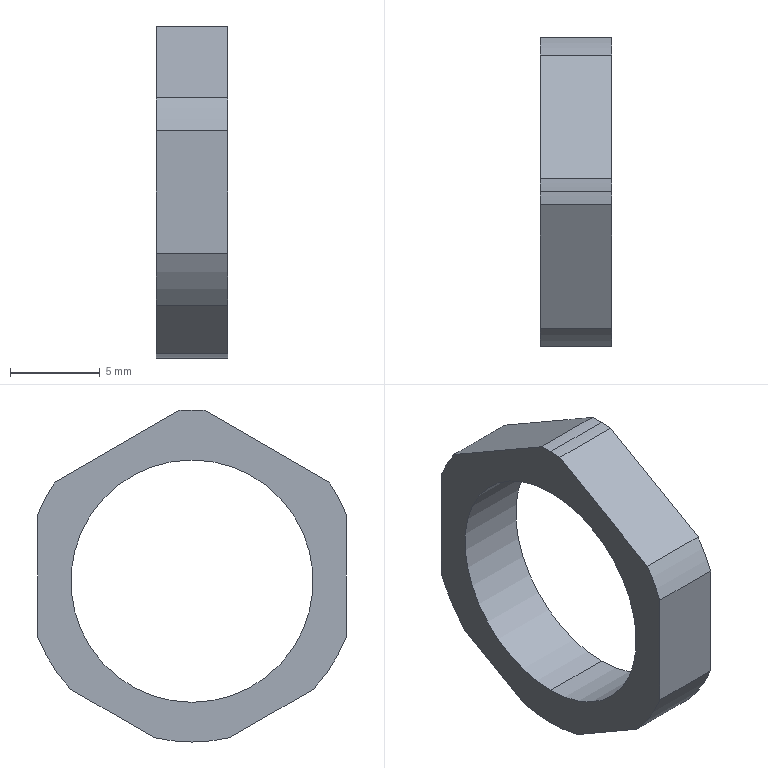Part | SolidWorks | features BaseBody 1 | 1 solid | 17 faces | box 4 x 17.2 x 18.5 mm | volume 428.753 mm3 | cylinder 9 | plane 8 | commonest cylinder face diameters 18.5 x7 13.5 x2
STEP:
#1=CARTESIAN_POINT('',(325.,17.5,16.75));
#2=VERTEX_POINT('',#1);
#3=CARTESIAN_POINT('',(325.,17.5,30.25));
#4=VERTEX_POINT('',#3);
#5=CARTESIAN_POINT('',(325.,17.5,23.5));
#6=DIRECTION('',(-1.,0.,0.));
#7=DIRECTION('',(0.,0.,1.));
#8=AXIS2_PLACEMENT_3D('',#5,#6,#7);
#9=CIRCLE('',#8,6.75);
#10=EDGE_CURVE('',#2,#4,#9,.T.);
#11=ORIENTED_EDGE('',*,*,#10,.F.);
#12=CARTESIAN_POINT('',(321.,17.5,16.75));
#13=VERTEX_POINT('',#12);
#14=CARTESIAN_POINT('',(325.,17.5,16.75));
#15=DIRECTION('',(-1.,0.,0.));
#16=VECTOR('',#15,1000.);
#17=LINE('',#14,#16);
#18=EDGE_CURVE('',#2,#13,#17,.T.);
#19=ORIENTED_EDGE('',*,*,#18,.T.);
#20=CARTESIAN_POINT('',(321.,17.5,30.25));
#21=VERTEX_POINT('',#20);
#22=CARTESIAN_POINT('',(321.,17.5,23.5));
#23=DIRECTION('',(-1.,0.,0.));
#24=DIRECTION('',(0.,0.,1.));
#25=AXIS2_PLACEMENT_3D('',#22,#23,#24);
#26=CIRCLE('',#25,6.75);
#27=EDGE_CURVE('',#13,#21,#26,.T.);
#28=ORIENTED_EDGE('',*,*,#27,.T.);
#29=CARTESIAN_POINT('',(325.,17.5,30.25));
#30=DIRECTION('',(-1.,0.,0.));
#31=VECTOR('',#30,1000.);
#32=LINE('',#29,#31);
#33=EDGE_CURVE('',#4,#21,#32,.T.);
#34=ORIENTED_EDGE('',*,*,#33,.F.);
#35=EDGE_LOOP('',(#11,#19,#28,#34));
#36=FACE_OUTER_BOUND('',#35,.T.);
#37=CARTESIAN_POINT('',(325.,17.5,23.5));
#38=DIRECTION('',(-1.,0.,0.));
#39=DIRECTION('',(0.,0.,1.));
#40=AXIS2_PLACEMENT_3D('',#37,#38,#39);
#41=CYLINDRICAL_SURFACE('',#40,6.75);
#42=ADVANCED_FACE('',(#36),#41,.F.);
#43=CARTESIAN_POINT('',(325.,17.5,33.038));
#44=VERTEX_POINT('',#43);
#45=CARTESIAN_POINT('',(325.,16.77,33.009));
#46=VERTEX_POINT('',#45);
#47=CARTESIAN_POINT('',(325.,17.5,23.788));
#48=DIRECTION('',(1.,0.,0.));
#49=DIRECTION('',(0.,0.,1.));
#50=AXIS2_PLACEMENT_3D('',#47,#48,#49);
#51=CIRCLE('',#50,9.25);
#52=EDGE_CURVE('',#44,#46,#51,.T.);
#53=ORIENTED_EDGE('',*,*,#52,.F.);
#54=CARTESIAN_POINT('',(321.,17.5,33.038));
#55=VERTEX_POINT('',#54);
#56=CARTESIAN_POINT('',(325.,17.5,33.038));
#57=DIRECTION('',(-1.,0.,0.));
#58=VECTOR('',#57,1000.);
#59=LINE('',#56,#58);
#60=EDGE_CURVE('',#44,#55,#59,.T.);
#61=ORIENTED_EDGE('',*,*,#60,.T.);
#62=CARTESIAN_POINT('',(321.,16.77,33.009));
#63=VERTEX_POINT('',#62);
#64=CARTESIAN_POINT('',(321.,17.5,23.788));
#65=DIRECTION('',(1.,0.,0.));
#66=DIRECTION('',(0.,0.,1.));
#67=AXIS2_PLACEMENT_3D('',#64,#65,#66);
#68=CIRCLE('',#67,9.25);
#69=EDGE_CURVE('',#55,#63,#68,.T.);
#70=ORIENTED_EDGE('',*,*,#69,.T.);
#71=CARTESIAN_POINT('',(325.,16.77,33.009));
#72=DIRECTION('',(1.,0.,0.));
#73=VECTOR('',#72,1000.);
#74=LINE('',#71,#73);
#75=EDGE_CURVE('',#63,#46,#74,.T.);
#76=ORIENTED_EDGE('',*,*,#75,.T.);
#77=EDGE_LOOP('',(#53,#61,#70,#76));
#78=FACE_OUTER_BOUND('',#77,.T.);
#79=CARTESIAN_POINT('',(325.,17.5,23.788));
#80=DIRECTION('',(-1.,0.,0.));
#81=DIRECTION('',(0.,0.,1.));
#82=AXIS2_PLACEMENT_3D('',#79,#80,#81);
#83=CYLINDRICAL_SURFACE('',#82,9.25);
#84=ADVANCED_FACE('',(#78),#83,.T.);
#85=CARTESIAN_POINT('',(325.,17.5,23.5));
#86=DIRECTION('',(-1.,0.,0.));
#87=DIRECTION('',(0.,0.,1.));
#88=AXIS2_PLACEMENT_3D('',#85,#86,#87);
#89=CIRCLE('',#88,6.75);
#90=EDGE_CURVE('',#4,#2,#89,.T.);
#91=ORIENTED_EDGE('',*,*,#90,.T.);
#92=ORIENTED_EDGE('',*,*,#10,.T.);
#93=EDGE_LOOP('',(#91,#92));
#94=FACE_BOUND('',#93,.T.);
#95=CARTESIAN_POINT('',(325.,25.121,29.03));
#96=VERTEX_POINT('',#95);
#97=CARTESIAN_POINT('',(325.,18.23,33.009));
#98=VERTEX_POINT('',#97);
#99=CARTESIAN_POINT('',(325.,25.121,29.03));
#100=DIRECTION('',(0.,-0.866,0.5));
#101=VECTOR('',#100,1000.);
#102=LINE('',#99,#101);
#103=EDGE_CURVE('',#96,#98,#102,.T.);
#104=ORIENTED_EDGE('',*,*,#103,.T.);
#105=CARTESIAN_POINT('',(325.,17.5,23.788));
#106=DIRECTION('',(1.,0.,0.));
#107=DIRECTION('',(0.,0.,1.));
#108=AXIS2_PLACEMENT_3D('',#105,#106,#107);
#109=CIRCLE('',#108,9.25);
#110=EDGE_CURVE('',#98,#44,#109,.T.);
#111=ORIENTED_EDGE('',*,*,#110,.T.);
#112=ORIENTED_EDGE('',*,*,#52,.T.);
#113=CARTESIAN_POINT('',(325.,9.879,29.03));
#114=VERTEX_POINT('',#113);
#115=CARTESIAN_POINT('',(325.,16.77,33.009));
#116=DIRECTION('',(0.,-0.866,-0.5));
#117=VECTOR('',#116,1000.);
#118=LINE('',#115,#117);
#119=EDGE_CURVE('',#46,#114,#118,.T.);
#120=ORIENTED_EDGE('',*,*,#119,.T.);
#121=CARTESIAN_POINT('',(325.,8.9,27.194));
#122=VERTEX_POINT('',#121);
#123=CARTESIAN_POINT('',(325.,17.5,23.788));
#124=DIRECTION('',(-1.,0.,0.));
#125=DIRECTION('',(0.,0.,1.));
#126=AXIS2_PLACEMENT_3D('',#123,#124,#125);
#127=CIRCLE('',#126,9.25);
#128=EDGE_CURVE('',#122,#114,#127,.T.);
#129=ORIENTED_EDGE('',*,*,#128,.F.);
#130=CARTESIAN_POINT('',(325.,8.9,20.382));
#131=VERTEX_POINT('',#130);
#132=CARTESIAN_POINT('',(325.,8.9,20.382));
#133=DIRECTION('',(0.,0.,1.));
#134=VECTOR('',#133,1000.);
#135=LINE('',#132,#134);
#136=EDGE_CURVE('',#131,#122,#135,.T.);
#137=ORIENTED_EDGE('',*,*,#136,.F.);
#138=CARTESIAN_POINT('',(325.,10.743,17.471));
#139=VERTEX_POINT('',#138);
#140=CARTESIAN_POINT('',(325.,17.5,23.788));
#141=DIRECTION('',(-1.,0.,0.));
#142=DIRECTION('',(0.,0.,1.));
#143=AXIS2_PLACEMENT_3D('',#140,#141,#142);
#144=CIRCLE('',#143,9.25);
#145=EDGE_CURVE('',#139,#131,#144,.T.);
#146=ORIENTED_EDGE('',*,*,#145,.F.);
#147=CARTESIAN_POINT('',(325.,15.407,14.778));
#148=VERTEX_POINT('',#147);
#149=CARTESIAN_POINT('',(325.,10.743,17.471));
#150=DIRECTION('',(0.,0.866,-0.5));
#151=VECTOR('',#150,1000.);
#152=LINE('',#149,#151);
#153=EDGE_CURVE('',#139,#148,#152,.T.);
#154=ORIENTED_EDGE('',*,*,#153,.T.);
#155=CARTESIAN_POINT('',(325.,19.593,14.778));
#156=VERTEX_POINT('',#155);
#157=CARTESIAN_POINT('',(325.,17.5,23.788));
#158=DIRECTION('',(-1.,0.,0.));
#159=DIRECTION('',(0.,0.,1.));
#160=AXIS2_PLACEMENT_3D('',#157,#158,#159);
#161=CIRCLE('',#160,9.25);
#162=EDGE_CURVE('',#156,#148,#161,.T.);
#163=ORIENTED_EDGE('',*,*,#162,.F.);
#164=CARTESIAN_POINT('',(325.,24.257,17.471));
#165=VERTEX_POINT('',#164);
#166=CARTESIAN_POINT('',(325.,19.593,14.778));
#167=DIRECTION('',(0.,0.866,0.5));
#168=VECTOR('',#167,1000.);
#169=LINE('',#166,#168);
#170=EDGE_CURVE('',#156,#165,#169,.T.);
#171=ORIENTED_EDGE('',*,*,#170,.T.);
#172=CARTESIAN_POINT('',(325.,26.1,20.382));
#173=VERTEX_POINT('',#172);
#174=CARTESIAN_POINT('',(325.,17.5,23.788));
#175=DIRECTION('',(-1.,0.,0.));
#176=DIRECTION('',(0.,0.,1.));
#177=AXIS2_PLACEMENT_3D('',#174,#175,#176);
#178=CIRCLE('',#177,9.25);
#179=EDGE_CURVE('',#173,#165,#178,.T.);
#180=ORIENTED_EDGE('',*,*,#179,.F.);
#181=CARTESIAN_POINT('',(325.,26.1,27.194));
#182=VERTEX_POINT('',#181);
#183=CARTESIAN_POINT('',(325.,26.1,27.194));
#184=DIRECTION('',(0.,0.,-1.));
#185=VECTOR('',#184,1000.);
#186=LINE('',#183,#185);
#187=EDGE_CURVE('',#182,#173,#186,.T.);
#188=ORIENTED_EDGE('',*,*,#187,.F.);
#189=CARTESIAN_POINT('',(325.,17.5,23.788));
#190=DIRECTION('',(-1.,0.,0.));
#191=DIRECTION('',(0.,0.,1.));
#192=AXIS2_PLACEMENT_3D('',#189,#190,#191);
#193=CIRCLE('',#192,9.25);
#194=EDGE_CURVE('',#96,#182,#193,.T.);
#195=ORIENTED_EDGE('',*,*,#194,.F.);
#196=EDGE_LOOP('',(#104,#111,#112,#120,#129,#137,#146,#154,#163,#171,#180,#188,#195));
#197=FACE_OUTER_BOUND('',#196,.T.);
#198=CARTESIAN_POINT('',(325.,17.5,23.5));
#199=DIRECTION('',(1.,0.,0.));
#200=DIRECTION('',(0.,1.,0.));
#201=AXIS2_PLACEMENT_3D('',#198,#199,#200);
#202=PLANE('',#201);
#203=ADVANCED_FACE('',(#94,#197),#202,.T.);
#204=CARTESIAN_POINT('',(321.,8.9,20.382));
#205=VERTEX_POINT('',#204);
#206=CARTESIAN_POINT('',(321.,10.743,17.471));
#207=VERTEX_POINT('',#206);
#208=CARTESIAN_POINT('',(321.,17.5,23.788));
#209=DIRECTION('',(1.,0.,0.));
#210=DIRECTION('',(0.,0.,1.));
#211=AXIS2_PLACEMENT_3D('',#208,#209,#210);
#212=CIRCLE('',#211,9.25);
#213=EDGE_CURVE('',#205,#207,#212,.T.);
#214=ORIENTED_EDGE('',*,*,#213,.T.);
#215=CARTESIAN_POINT('',(325.,10.743,17.471));
#216=DIRECTION('',(1.,0.,0.));
#217=VECTOR('',#216,1000.);
#218=LINE('',#215,#217);
#219=EDGE_CURVE('',#207,#139,#218,.T.);
#220=ORIENTED_EDGE('',*,*,#219,.T.);
#221=ORIENTED_EDGE('',*,*,#145,.T.);
#222=CARTESIAN_POINT('',(325.,8.9,20.382));
#223=DIRECTION('',(1.,0.,0.));
#224=VECTOR('',#223,1000.);
#225=LINE('',#222,#224);
#226=EDGE_CURVE('',#205,#131,#225,.T.);
#227=ORIENTED_EDGE('',*,*,#226,.F.);
#228=EDGE_LOOP('',(#214,#220,#221,#227));
#229=FACE_OUTER_BOUND('',#228,.T.);
#230=CARTESIAN_POINT('',(325.,17.5,23.788));
#231=DIRECTION('',(-1.,0.,0.));
#232=DIRECTION('',(0.,0.,1.));
#233=AXIS2_PLACEMENT_3D('',#230,#231,#232);
#234=CYLINDRICAL_SURFACE('',#233,9.25);
#235=ADVANCED_FACE('',(#229),#234,.T.);
#236=ORIENTED_EDGE('',*,*,#153,.F.);
#237=ORIENTED_EDGE('',*,*,#219,.F.);
#238=CARTESIAN_POINT('',(321.,15.407,14.778));
#239=VERTEX_POINT('',#238);
#240=CARTESIAN_POINT('',(321.,10.743,17.471));
#241=DIRECTION('',(0.,0.866,-0.5));
#242=VECTOR('',#241,1000.);
#243=LINE('',#240,#242);
#244=EDGE_CURVE('',#207,#239,#243,.T.);
#245=ORIENTED_EDGE('',*,*,#244,.T.);
#246=CARTESIAN_POINT('',(325.,15.407,14.778));
#247=DIRECTION('',(-1.,0.,0.));
#248=VECTOR('',#247,1000.);
#249=LINE('',#246,#248);
#250=EDGE_CURVE('',#148,#239,#249,.T.);
#251=ORIENTED_EDGE('',*,*,#250,.F.);
#252=EDGE_LOOP('',(#236,#237,#245,#251));
#253=FACE_OUTER_BOUND('',#252,.T.);
#254=CARTESIAN_POINT('',(325.,10.743,17.471));
#255=DIRECTION('',(0.,0.5,0.866));
#256=DIRECTION('',(1.,0.,0.));
#257=AXIS2_PLACEMENT_3D('',#254,#255,#256);
#258=PLANE('',#257);
#259=ADVANCED_FACE('',(#253),#258,.F.);
#260=ORIENTED_EDGE('',*,*,#162,.T.);
#261=ORIENTED_EDGE('',*,*,#250,.T.);
#262=CARTESIAN_POINT('',(321.,19.593,14.778));
#263=VERTEX_POINT('',#262);
#264=CARTESIAN_POINT('',(321.,17.5,23.788));
#265=DIRECTION('',(1.,0.,0.));
#266=DIRECTION('',(0.,0.,1.));
#267=AXIS2_PLACEMENT_3D('',#264,#265,#266);
#268=CIRCLE('',#267,9.25);
#269=EDGE_CURVE('',#239,#263,#268,.T.);
#270=ORIENTED_EDGE('',*,*,#269,.T.);
#271=CARTESIAN_POINT('',(325.,19.593,14.778));
#272=DIRECTION('',(1.,0.,0.));
#273=VECTOR('',#272,1000.);
#274=LINE('',#271,#273);
#275=EDGE_CURVE('',#263,#156,#274,.T.);
#276=ORIENTED_EDGE('',*,*,#275,.T.);
#277=EDGE_LOOP('',(#260,#261,#270,#276));
#278=FACE_OUTER_BOUND('',#277,.T.);
#279=CARTESIAN_POINT('',(325.,17.5,23.788));
#280=DIRECTION('',(-1.,0.,0.));
#281=DIRECTION('',(0.,0.,1.));
#282=AXIS2_PLACEMENT_3D('',#279,#280,#281);
#283=CYLINDRICAL_SURFACE('',#282,9.25);
#284=ADVANCED_FACE('',(#278),#283,.T.);
#285=ORIENTED_EDGE('',*,*,#170,.F.);
#286=ORIENTED_EDGE('',*,*,#275,.F.);
#287=CARTESIAN_POINT('',(321.,24.257,17.471));
#288=VERTEX_POINT('',#287);
#289=CARTESIAN_POINT('',(321.,19.593,14.778));
#290=DIRECTION('',(0.,0.866,0.5));
#291=VECTOR('',#290,1000.);
#292=LINE('',#289,#291);
#293=EDGE_CURVE('',#263,#288,#292,.T.);
#294=ORIENTED_EDGE('',*,*,#293,.T.);
#295=CARTESIAN_POINT('',(325.,24.257,17.471));
#296=DIRECTION('',(-1.,0.,0.));
#297=VECTOR('',#296,1000.);
#298=LINE('',#295,#297);
#299=EDGE_CURVE('',#165,#288,#298,.T.);
#300=ORIENTED_EDGE('',*,*,#299,.F.);
#301=EDGE_LOOP('',(#285,#286,#294,#300));
#302=FACE_OUTER_BOUND('',#301,.T.);
#303=CARTESIAN_POINT('',(325.,19.593,14.778));
#304=DIRECTION('',(0.,-0.5,0.866));
#305=DIRECTION('',(-1.,0.,0.));
#306=AXIS2_PLACEMENT_3D('',#303,#304,#305);
#307=PLANE('',#306);
#308=ADVANCED_FACE('',(#302),#307,.F.);
#309=CARTESIAN_POINT('',(321.,26.1,20.382));
#310=VERTEX_POINT('',#309);
#311=CARTESIAN_POINT('',(321.,17.5,23.788));
#312=DIRECTION('',(1.,0.,0.));
#313=DIRECTION('',(0.,0.,1.));
#314=AXIS2_PLACEMENT_3D('',#311,#312,#313);
#315=CIRCLE('',#314,9.25);
#316=EDGE_CURVE('',#288,#310,#315,.T.);
#317=ORIENTED_EDGE('',*,*,#316,.T.);
#318=CARTESIAN_POINT('',(325.,26.1,20.382));
#319=DIRECTION('',(-1.,0.,0.));
#320=VECTOR('',#319,1000.);
#321=LINE('',#318,#320);
#322=EDGE_CURVE('',#173,#310,#321,.T.);
#323=ORIENTED_EDGE('',*,*,#322,.F.);
#324=ORIENTED_EDGE('',*,*,#179,.T.);
#325=ORIENTED_EDGE('',*,*,#299,.T.);
#326=EDGE_LOOP('',(#317,#323,#324,#325));
#327=FACE_OUTER_BOUND('',#326,.T.);
#328=CARTESIAN_POINT('',(325.,17.5,23.788));
#329=DIRECTION('',(-1.,0.,0.));
#330=DIRECTION('',(0.,0.,1.));
#331=AXIS2_PLACEMENT_3D('',#328,#329,#330);
#332=CYLINDRICAL_SURFACE('',#331,9.25);
#333=ADVANCED_FACE('',(#327),#332,.T.);
#334=CARTESIAN_POINT('',(321.,26.1,27.194));
#335=VERTEX_POINT('',#334);
#336=CARTESIAN_POINT('',(321.,26.1,23.5));
#337=DIRECTION('',(0.,0.,1.));
#338=VECTOR('',#337,1000.);
#339=LINE('',#336,#338);
#340=EDGE_CURVE('',#310,#335,#339,.T.);
#341=ORIENTED_EDGE('',*,*,#340,.T.);
#342=CARTESIAN_POINT('',(325.,26.1,27.194));
#343=DIRECTION('',(-1.,0.,0.));
#344=VECTOR('',#343,1000.);
#345=LINE('',#342,#344);
#346=EDGE_CURVE('',#182,#335,#345,.T.);
#347=ORIENTED_EDGE('',*,*,#346,.F.);
#348=ORIENTED_EDGE('',*,*,#187,.T.);
#349=ORIENTED_EDGE('',*,*,#322,.T.);
#350=EDGE_LOOP('',(#341,#347,#348,#349));
#351=FACE_OUTER_BOUND('',#350,.T.);
#352=CARTESIAN_POINT('',(325.,26.1,27.194));
#353=DIRECTION('',(0.,1.,0.));
#354=DIRECTION('',(1.,0.,0.));
#355=AXIS2_PLACEMENT_3D('',#352,#353,#354);
#356=PLANE('',#355);
#357=ADVANCED_FACE('',(#351),#356,.T.);
#358=CARTESIAN_POINT('',(321.,25.121,29.03));
#359=VERTEX_POINT('',#358);
#360=CARTESIAN_POINT('',(321.,17.5,23.788));
#361=DIRECTION('',(1.,0.,0.));
#362=DIRECTION('',(0.,0.,1.));
#363=AXIS2_PLACEMENT_3D('',#360,#361,#362);
#364=CIRCLE('',#363,9.25);
#365=EDGE_CURVE('',#335,#359,#364,.T.);
#366=ORIENTED_EDGE('',*,*,#365,.T.);
#367=CARTESIAN_POINT('',(325.,25.121,29.03));
#368=DIRECTION('',(1.,0.,0.));
#369=VECTOR('',#368,1000.);
#370=LINE('',#367,#369);
#371=EDGE_CURVE('',#359,#96,#370,.T.);
#372=ORIENTED_EDGE('',*,*,#371,.T.);
#373=ORIENTED_EDGE('',*,*,#194,.T.);
#374=ORIENTED_EDGE('',*,*,#346,.T.);
#375=EDGE_LOOP('',(#366,#372,#373,#374));
#376=FACE_OUTER_BOUND('',#375,.T.);
#377=CARTESIAN_POINT('',(325.,17.5,23.788));
#378=DIRECTION('',(-1.,0.,0.));
#379=DIRECTION('',(0.,0.,1.));
#380=AXIS2_PLACEMENT_3D('',#377,#378,#379);
#381=CYLINDRICAL_SURFACE('',#380,9.25);
#382=ADVANCED_FACE('',(#376),#381,.T.);
#383=ORIENTED_EDGE('',*,*,#103,.F.);
#384=ORIENTED_EDGE('',*,*,#371,.F.);
#385=CARTESIAN_POINT('',(321.,18.23,33.009));
#386=VERTEX_POINT('',#385);
#387=CARTESIAN_POINT('',(321.,25.121,29.03));
#388=DIRECTION('',(0.,-0.866,0.5));
#389=VECTOR('',#388,1000.);
#390=LINE('',#387,#389);
#391=EDGE_CURVE('',#359,#386,#390,.T.);
#392=ORIENTED_EDGE('',*,*,#391,.T.);
#393=CARTESIAN_POINT('',(325.,18.23,33.009));
#394=DIRECTION('',(-1.,0.,0.));
#395=VECTOR('',#394,1000.);
#396=LINE('',#393,#395);
#397=EDGE_CURVE('',#98,#386,#396,.T.);
#398=ORIENTED_EDGE('',*,*,#397,.F.);
#399=EDGE_LOOP('',(#383,#384,#392,#398));
#400=FACE_OUTER_BOUND('',#399,.T.);
#401=CARTESIAN_POINT('',(325.,25.121,29.03));
#402=DIRECTION('',(0.,-0.5,-0.866));
#403=DIRECTION('',(0.,-0.866,0.5));
#404=AXIS2_PLACEMENT_3D('',#401,#402,#403);
#405=PLANE('',#404);
#406=ADVANCED_FACE('',(#400),#405,.F.);
#407=ORIENTED_EDGE('',*,*,#119,.F.);
#408=ORIENTED_EDGE('',*,*,#75,.F.);
#409=CARTESIAN_POINT('',(321.,9.879,29.03));
#410=VERTEX_POINT('',#409);
#411=CARTESIAN_POINT('',(321.,16.77,33.009));
#412=DIRECTION('',(0.,-0.866,-0.5));
#413=VECTOR('',#412,1000.);
#414=LINE('',#411,#413);
#415=EDGE_CURVE('',#63,#410,#414,.T.);
#416=ORIENTED_EDGE('',*,*,#415,.T.);
#417=CARTESIAN_POINT('',(325.,9.879,29.03));
#418=DIRECTION('',(-1.,0.,0.));
#419=VECTOR('',#418,1000.);
#420=LINE('',#417,#419);
#421=EDGE_CURVE('',#114,#410,#420,.T.);
#422=ORIENTED_EDGE('',*,*,#421,.F.);
#423=EDGE_LOOP('',(#407,#408,#416,#422));
#424=FACE_OUTER_BOUND('',#423,.T.);
#425=CARTESIAN_POINT('',(325.,16.77,33.009));
#426=DIRECTION('',(0.,0.5,-0.866));
#427=DIRECTION('',(-1.,0.,0.));
#428=AXIS2_PLACEMENT_3D('',#425,#426,#427);
#429=PLANE('',#428);
#430=ADVANCED_FACE('',(#424),#429,.F.);
#431=CARTESIAN_POINT('',(321.,8.9,27.194));
#432=VERTEX_POINT('',#431);
#433=CARTESIAN_POINT('',(321.,17.5,23.788));
#434=DIRECTION('',(1.,0.,0.));
#435=DIRECTION('',(0.,0.,1.));
#436=AXIS2_PLACEMENT_3D('',#433,#434,#435);
#437=CIRCLE('',#436,9.25);
#438=EDGE_CURVE('',#410,#432,#437,.T.);
#439=ORIENTED_EDGE('',*,*,#438,.T.);
#440=CARTESIAN_POINT('',(325.,8.9,27.194));
#441=DIRECTION('',(-1.,0.,0.));
#442=VECTOR('',#441,1000.);
#443=LINE('',#440,#442);
#444=EDGE_CURVE('',#122,#432,#443,.T.);
#445=ORIENTED_EDGE('',*,*,#444,.F.);
#446=ORIENTED_EDGE('',*,*,#128,.T.);
#447=ORIENTED_EDGE('',*,*,#421,.T.);
#448=EDGE_LOOP('',(#439,#445,#446,#447));
#449=FACE_OUTER_BOUND('',#448,.T.);
#450=CARTESIAN_POINT('',(325.,17.5,23.788));
#451=DIRECTION('',(-1.,0.,0.));
#452=DIRECTION('',(0.,0.,1.));
#453=AXIS2_PLACEMENT_3D('',#450,#451,#452);
#454=CYLINDRICAL_SURFACE('',#453,9.25);
#455=ADVANCED_FACE('',(#449),#454,.T.);
#456=CARTESIAN_POINT('',(321.,8.9,23.5));
#457=DIRECTION('',(0.,0.,-1.));
#458=VECTOR('',#457,1000.);
#459=LINE('',#456,#458);
#460=EDGE_CURVE('',#432,#205,#459,.T.);
#461=ORIENTED_EDGE('',*,*,#460,.T.);
#462=ORIENTED_EDGE('',*,*,#226,.T.);
#463=ORIENTED_EDGE('',*,*,#136,.T.);
#464=ORIENTED_EDGE('',*,*,#444,.T.);
#465=EDGE_LOOP('',(#461,#462,#463,#464));
#466=FACE_OUTER_BOUND('',#465,.T.);
#467=CARTESIAN_POINT('',(325.,8.9,20.382));
#468=DIRECTION('',(0.,-1.,0.));
#469=DIRECTION('',(0.,0.,-1.));
#470=AXIS2_PLACEMENT_3D('',#467,#468,#469);
#471=PLANE('',#470);
#472=ADVANCED_FACE('',(#466),#471,.T.);
#473=CARTESIAN_POINT('',(321.,17.5,23.5));
#474=DIRECTION('',(-1.,0.,0.));
#475=DIRECTION('',(0.,0.,1.));
#476=AXIS2_PLACEMENT_3D('',#473,#474,#475);
#477=CIRCLE('',#476,6.75);
#478=EDGE_CURVE('',#21,#13,#477,.T.);
#479=ORIENTED_EDGE('',*,*,#478,.F.);
#480=ORIENTED_EDGE('',*,*,#27,.F.);
#481=EDGE_LOOP('',(#479,#480));
#482=FACE_BOUND('',#481,.T.);
#483=ORIENTED_EDGE('',*,*,#438,.F.);
#484=ORIENTED_EDGE('',*,*,#415,.F.);
#485=ORIENTED_EDGE('',*,*,#69,.F.);
#486=CARTESIAN_POINT('',(321.,17.5,23.788));
#487=DIRECTION('',(1.,0.,0.));
#488=DIRECTION('',(0.,0.,1.));
#489=AXIS2_PLACEMENT_3D('',#486,#487,#488);
#490=CIRCLE('',#489,9.25);
#491=EDGE_CURVE('',#386,#55,#490,.T.);
#492=ORIENTED_EDGE('',*,*,#491,.F.);
#493=ORIENTED_EDGE('',*,*,#391,.F.);
#494=ORIENTED_EDGE('',*,*,#365,.F.);
#495=ORIENTED_EDGE('',*,*,#340,.F.);
#496=ORIENTED_EDGE('',*,*,#316,.F.);
#497=ORIENTED_EDGE('',*,*,#293,.F.);
#498=ORIENTED_EDGE('',*,*,#269,.F.);
#499=ORIENTED_EDGE('',*,*,#244,.F.);
#500=ORIENTED_EDGE('',*,*,#213,.F.);
#501=ORIENTED_EDGE('',*,*,#460,.F.);
#502=EDGE_LOOP('',(#483,#484,#485,#492,#493,#494,#495,#496,#497,#498,#499,#500,#501));
#503=FACE_OUTER_BOUND('',#502,.T.);
#504=CARTESIAN_POINT('',(321.,17.5,23.5));
#505=DIRECTION('',(1.,0.,0.));
#506=DIRECTION('',(0.,1.,0.));
#507=AXIS2_PLACEMENT_3D('',#504,#505,#506);
#508=PLANE('',#507);
#509=ADVANCED_FACE('',(#482,#503),#508,.F.);
#510=ORIENTED_EDGE('',*,*,#60,.F.);
#511=ORIENTED_EDGE('',*,*,#110,.F.);
#512=ORIENTED_EDGE('',*,*,#397,.T.);
#513=ORIENTED_EDGE('',*,*,#491,.T.);
#514=EDGE_LOOP('',(#510,#511,#512,#513));
#515=FACE_OUTER_BOUND('',#514,.T.);
#516=CARTESIAN_POINT('',(325.,17.5,23.788));
#517=DIRECTION('',(-1.,0.,0.));
#518=DIRECTION('',(0.,0.,1.));
#519=AXIS2_PLACEMENT_3D('',#516,#517,#518);
#520=CYLINDRICAL_SURFACE('',#519,9.25);
#521=ADVANCED_FACE('',(#515),#520,.T.);
#522=ORIENTED_EDGE('',*,*,#18,.F.);
#523=ORIENTED_EDGE('',*,*,#90,.F.);
#524=ORIENTED_EDGE('',*,*,#33,.T.);
#525=ORIENTED_EDGE('',*,*,#478,.T.);
#526=EDGE_LOOP('',(#522,#523,#524,#525));
#527=FACE_OUTER_BOUND('',#526,.T.);
#528=CARTESIAN_POINT('',(325.,17.5,23.5));
#529=DIRECTION('',(-1.,0.,0.));
#530=DIRECTION('',(0.,0.,1.));
#531=AXIS2_PLACEMENT_3D('',#528,#529,#530);
#532=CYLINDRICAL_SURFACE('',#531,6.75);
#533=ADVANCED_FACE('',(#527),#532,.F.);
#534=CLOSED_SHELL('',(#42,#84,#203,#235,#259,#284,#308,#333,#357,#382,#406,#430,#455,#472,#509,#521,#533));
#535=MANIFOLD_SOLID_BREP('',#534);
#536=CARTESIAN_POINT('',(0.,0.,0.));
#537=DIRECTION('',(0.,0.,1.));
#538=DIRECTION('',(1.,0.,0.));
#539=AXIS2_PLACEMENT_3D('',#536,#537,#538);
#540=(LENGTH_UNIT()NAMED_UNIT(*)SI_UNIT(.MILLI.,.METRE.));
#541=UNCERTAINTY_MEASURE_WITH_UNIT(LENGTH_MEASURE(0.00001),#540,'','');
#542=(NAMED_UNIT(*)PLANE_ANGLE_UNIT()SI_UNIT($,.RADIAN.));
#543=(NAMED_UNIT(*)SI_UNIT($,.STERADIAN.)SOLID_ANGLE_UNIT());
#544=(GEOMETRIC_REPRESENTATION_CONTEXT(3)GLOBAL_UNCERTAINTY_ASSIGNED_CONTEXT((#541))GLOBAL_UNIT_ASSIGNED_CONTEXT((#540,#542,#543))REPRESENTATION_CONTEXT('',''));
#545=ADVANCED_BREP_SHAPE_REPRESENTATION('',(#535,#539),#544);